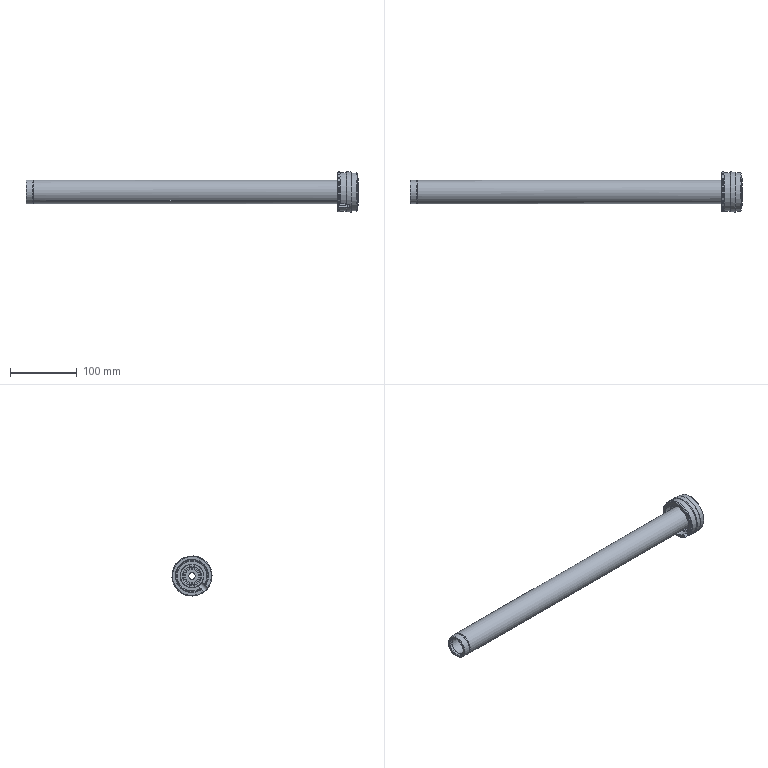Part | STEP file | Nozzle Body(02) | 1 solid | 57 faces | box 497 x 60 x 60 mm | volume 469077 mm3 | plane 23 | cylinder 20 | cone 10 | torus 4 | commonest cylinder face diameters 35.3 x2 58 x2 60 x2 1 x1 1.7 x1 8 x1